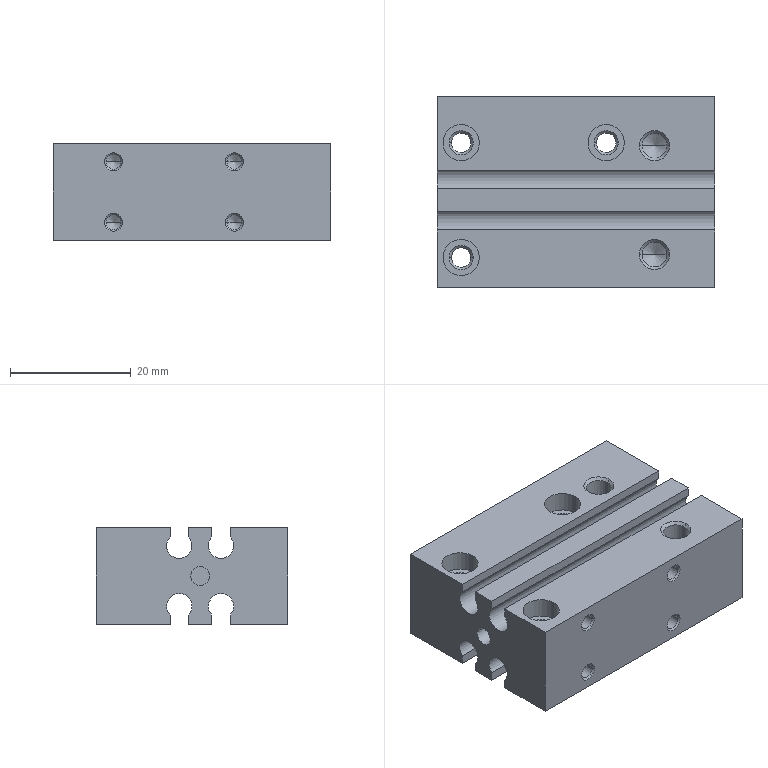Part | STEP file | MXH6-15-a | 1 solid | 150 faces | box 46 x 31.7 x 16 mm | volume 17954 mm3 | cone 68 | cylinder 56 | plane 26 | commonest cylinder face diameters 2.459 x16 6 x14 4.134 x12 3.242 x6 4.2 x6 3.1 x2